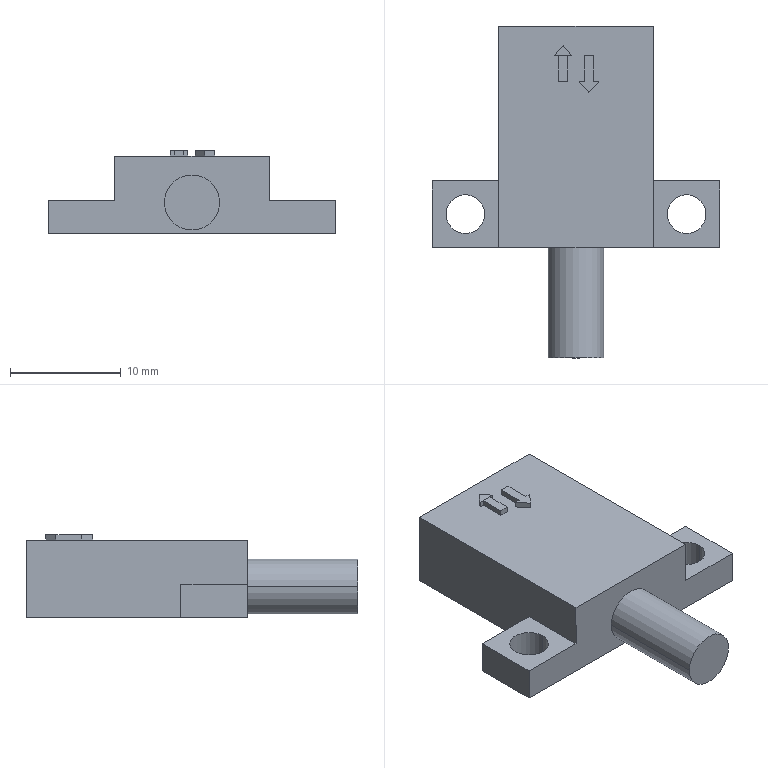Part | NX | features BREP 1 | 1 solid | 41 faces | box 26 x 30 x 7.5 mm | volume 2301 mm3 | plane 35 | cylinder 6 | commonest cylinder face diameters 3.5 x4 5 x2
STEP:
#1=CARTESIAN_POINT('',(4.,19.5,5.5));
#2=VERTEX_POINT('',#1);
#3=CARTESIAN_POINT('',(4.,19.5,1.5));
#4=VERTEX_POINT('',#3);
#5=CARTESIAN_POINT('',(4.,19.5,5.5));
#6=DIRECTION('',(0.,0.,-1.));
#7=VECTOR('',#6,1000.);
#8=LINE('',#5,#7);
#9=EDGE_CURVE('',#2,#4,#8,.T.);
#10=ORIENTED_EDGE('',*,*,#9,.T.);
#11=CARTESIAN_POINT('',(-4.,19.5,1.5));
#12=VERTEX_POINT('',#11);
#13=CARTESIAN_POINT('',(-4.,19.5,1.5));
#14=DIRECTION('',(-1.,0.,0.));
#15=VECTOR('',#14,1000.);
#16=LINE('',#13,#15);
#17=EDGE_CURVE('',#4,#12,#16,.T.);
#18=ORIENTED_EDGE('',*,*,#17,.T.);
#19=CARTESIAN_POINT('',(-4.,19.5,5.5));
#20=VERTEX_POINT('',#19);
#21=CARTESIAN_POINT('',(-4.,19.5,5.5));
#22=DIRECTION('',(0.,0.,1.));
#23=VECTOR('',#22,1000.);
#24=LINE('',#21,#23);
#25=EDGE_CURVE('',#12,#20,#24,.T.);
#26=ORIENTED_EDGE('',*,*,#25,.T.);
#27=CARTESIAN_POINT('',(-4.,19.5,5.5));
#28=DIRECTION('',(1.,0.,0.));
#29=VECTOR('',#28,1000.);
#30=LINE('',#27,#29);
#31=EDGE_CURVE('',#20,#2,#30,.T.);
#32=ORIENTED_EDGE('',*,*,#31,.T.);
#33=EDGE_LOOP('',(#10,#18,#26,#32));
#34=FACE_BOUND('',#33,.T.);
#35=CARTESIAN_POINT('',(0.,19.5,0.));
#36=DIRECTION('',(0.,-1.,0.));
#37=DIRECTION('',(0.,0.,-1.));
#38=AXIS2_PLACEMENT_3D('',#35,#36,#37);
#39=PLANE('',#38);
#40=ADVANCED_FACE('',(#34),#39,.F.);
#41=CARTESIAN_POINT('',(4.,20.,1.5));
#42=VERTEX_POINT('',#41);
#43=CARTESIAN_POINT('',(-4.,20.,1.5));
#44=VERTEX_POINT('',#43);
#45=CARTESIAN_POINT('',(-4.,20.,1.5));
#46=DIRECTION('',(-1.,0.,0.));
#47=VECTOR('',#46,1000.);
#48=LINE('',#45,#47);
#49=EDGE_CURVE('',#42,#44,#48,.T.);
#50=ORIENTED_EDGE('',*,*,#49,.T.);
#51=CARTESIAN_POINT('',(-4.,19.5,1.5));
#52=DIRECTION('',(0.,1.,0.));
#53=VECTOR('',#52,1000.);
#54=LINE('',#51,#53);
#55=EDGE_CURVE('',#12,#44,#54,.T.);
#56=ORIENTED_EDGE('',*,*,#55,.F.);
#57=ORIENTED_EDGE('',*,*,#17,.F.);
#58=CARTESIAN_POINT('',(4.,19.5,1.5));
#59=DIRECTION('',(0.,1.,0.));
#60=VECTOR('',#59,1000.);
#61=LINE('',#58,#60);
#62=EDGE_CURVE('',#4,#42,#61,.T.);
#63=ORIENTED_EDGE('',*,*,#62,.T.);
#64=EDGE_LOOP('',(#50,#56,#57,#63));
#65=FACE_BOUND('',#64,.T.);
#66=CARTESIAN_POINT('',(-4.,19.5,1.5));
#67=DIRECTION('',(0.,0.,-1.));
#68=DIRECTION('',(-1.,0.,0.));
#69=AXIS2_PLACEMENT_3D('',#66,#67,#68);
#70=PLANE('',#69);
#71=ADVANCED_FACE('',(#65),#70,.F.);
#72=CARTESIAN_POINT('',(-4.,20.,5.5));
#73=VERTEX_POINT('',#72);
#74=CARTESIAN_POINT('',(-4.,20.,5.5));
#75=DIRECTION('',(0.,0.,1.));
#76=VECTOR('',#75,1000.);
#77=LINE('',#74,#76);
#78=EDGE_CURVE('',#44,#73,#77,.T.);
#79=ORIENTED_EDGE('',*,*,#78,.T.);
#80=CARTESIAN_POINT('',(-4.,19.5,5.5));
#81=DIRECTION('',(0.,1.,0.));
#82=VECTOR('',#81,1000.);
#83=LINE('',#80,#82);
#84=EDGE_CURVE('',#20,#73,#83,.T.);
#85=ORIENTED_EDGE('',*,*,#84,.F.);
#86=ORIENTED_EDGE('',*,*,#25,.F.);
#87=ORIENTED_EDGE('',*,*,#55,.T.);
#88=EDGE_LOOP('',(#79,#85,#86,#87));
#89=FACE_BOUND('',#88,.T.);
#90=CARTESIAN_POINT('',(-4.,19.5,5.5));
#91=DIRECTION('',(-1.,0.,0.));
#92=DIRECTION('',(0.,0.,1.));
#93=AXIS2_PLACEMENT_3D('',#90,#91,#92);
#94=PLANE('',#93);
#95=ADVANCED_FACE('',(#89),#94,.F.);
#96=CARTESIAN_POINT('',(4.,20.,5.5));
#97=VERTEX_POINT('',#96);
#98=CARTESIAN_POINT('',(-4.,20.,5.5));
#99=DIRECTION('',(1.,0.,0.));
#100=VECTOR('',#99,1000.);
#101=LINE('',#98,#100);
#102=EDGE_CURVE('',#73,#97,#101,.T.);
#103=ORIENTED_EDGE('',*,*,#102,.T.);
#104=CARTESIAN_POINT('',(4.,19.5,5.5));
#105=DIRECTION('',(0.,1.,0.));
#106=VECTOR('',#105,1000.);
#107=LINE('',#104,#106);
#108=EDGE_CURVE('',#2,#97,#107,.T.);
#109=ORIENTED_EDGE('',*,*,#108,.F.);
#110=ORIENTED_EDGE('',*,*,#31,.F.);
#111=ORIENTED_EDGE('',*,*,#84,.T.);
#112=EDGE_LOOP('',(#103,#109,#110,#111));
#113=FACE_BOUND('',#112,.T.);
#114=CARTESIAN_POINT('',(-4.,19.5,5.5));
#115=DIRECTION('',(0.,0.,1.));
#116=DIRECTION('',(1.,0.,0.));
#117=AXIS2_PLACEMENT_3D('',#114,#115,#116);
#118=PLANE('',#117);
#119=ADVANCED_FACE('',(#113),#118,.F.);
#120=CARTESIAN_POINT('',(4.,20.,5.5));
#121=DIRECTION('',(0.,0.,-1.));
#122=VECTOR('',#121,1000.);
#123=LINE('',#120,#122);
#124=EDGE_CURVE('',#97,#42,#123,.T.);
#125=ORIENTED_EDGE('',*,*,#124,.T.);
#126=ORIENTED_EDGE('',*,*,#62,.F.);
#127=ORIENTED_EDGE('',*,*,#9,.F.);
#128=ORIENTED_EDGE('',*,*,#108,.T.);
#129=EDGE_LOOP('',(#125,#126,#127,#128));
#130=FACE_BOUND('',#129,.T.);
#131=CARTESIAN_POINT('',(4.,19.5,5.5));
#132=DIRECTION('',(1.,0.,0.));
#133=DIRECTION('',(0.,0.,-1.));
#134=AXIS2_PLACEMENT_3D('',#131,#132,#133);
#135=PLANE('',#134);
#136=ADVANCED_FACE('',(#130),#135,.F.);
#137=CARTESIAN_POINT('',(-2.5,-10.,2.8));
#138=VERTEX_POINT('',#137);
#139=CARTESIAN_POINT('',(2.5,-10.,2.8));
#140=VERTEX_POINT('',#139);
#141=CARTESIAN_POINT('',(0.,-10.,2.8));
#142=DIRECTION('',(0.,-1.,0.));
#143=DIRECTION('',(1.,0.,0.));
#144=AXIS2_PLACEMENT_3D('',#141,#142,#143);
#145=CIRCLE('',#144,2.5);
#146=EDGE_CURVE('',#138,#140,#145,.T.);
#147=ORIENTED_EDGE('',*,*,#146,.T.);
#148=CARTESIAN_POINT('',(0.,-10.,2.8));
#149=DIRECTION('',(0.,-1.,0.));
#150=DIRECTION('',(1.,0.,0.));
#151=AXIS2_PLACEMENT_3D('',#148,#149,#150);
#152=CIRCLE('',#151,2.5);
#153=EDGE_CURVE('',#140,#138,#152,.T.);
#154=ORIENTED_EDGE('',*,*,#153,.T.);
#155=EDGE_LOOP('',(#147,#154));
#156=FACE_BOUND('',#155,.T.);
#157=CARTESIAN_POINT('',(0.,-10.,2.8));
#158=DIRECTION('',(0.,-1.,0.));
#159=DIRECTION('',(1.,0.,0.));
#160=AXIS2_PLACEMENT_3D('',#157,#158,#159);
#161=PLANE('',#160);
#162=ADVANCED_FACE('',(#156),#161,.T.);
#163=CARTESIAN_POINT('',(2.5,0.,2.8));
#164=VERTEX_POINT('',#163);
#165=CARTESIAN_POINT('',(2.5,-10.,2.8));
#166=DIRECTION('',(0.,1.,0.));
#167=VECTOR('',#166,1000.);
#168=LINE('',#165,#167);
#169=EDGE_CURVE('',#140,#164,#168,.T.);
#170=ORIENTED_EDGE('',*,*,#169,.F.);
#171=ORIENTED_EDGE('',*,*,#146,.F.);
#172=CARTESIAN_POINT('',(-2.5,0.,2.8));
#173=VERTEX_POINT('',#172);
#174=CARTESIAN_POINT('',(-2.5,-10.,2.8));
#175=DIRECTION('',(0.,1.,0.));
#176=VECTOR('',#175,1000.);
#177=LINE('',#174,#176);
#178=EDGE_CURVE('',#138,#173,#177,.T.);
#179=ORIENTED_EDGE('',*,*,#178,.T.);
#180=CARTESIAN_POINT('',(0.,0.,2.8));
#181=DIRECTION('',(0.,-1.,0.));
#182=DIRECTION('',(-1.,0.,0.));
#183=AXIS2_PLACEMENT_3D('',#180,#181,#182);
#184=CIRCLE('',#183,2.5);
#185=EDGE_CURVE('',#173,#164,#184,.T.);
#186=ORIENTED_EDGE('',*,*,#185,.T.);
#187=EDGE_LOOP('',(#170,#171,#179,#186));
#188=FACE_BOUND('',#187,.T.);
#189=CARTESIAN_POINT('',(0.,-10.,2.8));
#190=DIRECTION('',(0.,1.,0.));
#191=DIRECTION('',(-1.,0.,0.));
#192=AXIS2_PLACEMENT_3D('',#189,#190,#191);
#193=CYLINDRICAL_SURFACE('',#192,2.5);
#194=ADVANCED_FACE('',(#188),#193,.T.);
#195=CARTESIAN_POINT('',(-11.75,3.,3.));
#196=VERTEX_POINT('',#195);
#197=CARTESIAN_POINT('',(-11.75,3.,0.));
#198=VERTEX_POINT('',#197);
#199=CARTESIAN_POINT('',(-11.75,3.,3.));
#200=DIRECTION('',(0.,0.,1.));
#201=VECTOR('',#200,1000.);
#202=LINE('',#199,#201);
#203=EDGE_CURVE('',#196,#198,#202,.F.);
#204=ORIENTED_EDGE('',*,*,#203,.T.);
#205=CARTESIAN_POINT('',(-8.25,3.,0.));
#206=VERTEX_POINT('',#205);
#207=CARTESIAN_POINT('',(-10.,3.,0.));
#208=DIRECTION('',(0.,0.,1.));
#209=DIRECTION('',(1.,0.,0.));
#210=AXIS2_PLACEMENT_3D('',#207,#208,#209);
#211=CIRCLE('',#210,1.75);
#212=EDGE_CURVE('',#206,#198,#211,.T.);
#213=ORIENTED_EDGE('',*,*,#212,.F.);
#214=CARTESIAN_POINT('',(-8.25,3.,3.));
#215=VERTEX_POINT('',#214);
#216=CARTESIAN_POINT('',(-8.25,3.,3.));
#217=DIRECTION('',(0.,0.,1.));
#218=VECTOR('',#217,1000.);
#219=LINE('',#216,#218);
#220=EDGE_CURVE('',#215,#206,#219,.F.);
#221=ORIENTED_EDGE('',*,*,#220,.F.);
#222=CARTESIAN_POINT('',(-10.,3.,3.));
#223=DIRECTION('',(0.,0.,1.));
#224=DIRECTION('',(1.,0.,0.));
#225=AXIS2_PLACEMENT_3D('',#222,#223,#224);
#226=CIRCLE('',#225,1.75);
#227=EDGE_CURVE('',#215,#196,#226,.T.);
#228=ORIENTED_EDGE('',*,*,#227,.T.);
#229=EDGE_LOOP('',(#204,#213,#221,#228));
#230=FACE_BOUND('',#229,.T.);
#231=CARTESIAN_POINT('',(-10.,3.,3.));
#232=DIRECTION('',(0.,0.,1.));
#233=DIRECTION('',(1.,0.,0.));
#234=AXIS2_PLACEMENT_3D('',#231,#232,#233);
#235=CYLINDRICAL_SURFACE('',#234,1.75);
#236=ADVANCED_FACE('',(#230),#235,.F.);
#237=CARTESIAN_POINT('',(8.25,3.,3.));
#238=VERTEX_POINT('',#237);
#239=CARTESIAN_POINT('',(8.25,3.,0.));
#240=VERTEX_POINT('',#239);
#241=CARTESIAN_POINT('',(8.25,3.,3.));
#242=DIRECTION('',(0.,0.,1.));
#243=VECTOR('',#242,1000.);
#244=LINE('',#241,#243);
#245=EDGE_CURVE('',#238,#240,#244,.F.);
#246=ORIENTED_EDGE('',*,*,#245,.T.);
#247=CARTESIAN_POINT('',(11.75,3.,0.));
#248=VERTEX_POINT('',#247);
#249=CARTESIAN_POINT('',(10.,3.,0.));
#250=DIRECTION('',(0.,0.,1.));
#251=DIRECTION('',(1.,0.,0.));
#252=AXIS2_PLACEMENT_3D('',#249,#250,#251);
#253=CIRCLE('',#252,1.75);
#254=EDGE_CURVE('',#248,#240,#253,.T.);
#255=ORIENTED_EDGE('',*,*,#254,.F.);
#256=CARTESIAN_POINT('',(11.75,3.,3.));
#257=VERTEX_POINT('',#256);
#258=CARTESIAN_POINT('',(11.75,3.,3.));
#259=DIRECTION('',(0.,0.,1.));
#260=VECTOR('',#259,1000.);
#261=LINE('',#258,#260);
#262=EDGE_CURVE('',#257,#248,#261,.F.);
#263=ORIENTED_EDGE('',*,*,#262,.F.);
#264=CARTESIAN_POINT('',(10.,3.,3.));
#265=DIRECTION('',(0.,0.,1.));
#266=DIRECTION('',(1.,0.,0.));
#267=AXIS2_PLACEMENT_3D('',#264,#265,#266);
#268=CIRCLE('',#267,1.75);
#269=EDGE_CURVE('',#257,#238,#268,.T.);
#270=ORIENTED_EDGE('',*,*,#269,.T.);
#271=EDGE_LOOP('',(#246,#255,#263,#270));
#272=FACE_BOUND('',#271,.T.);
#273=CARTESIAN_POINT('',(10.,3.,3.));
#274=DIRECTION('',(0.,0.,1.));
#275=DIRECTION('',(1.,0.,0.));
#276=AXIS2_PLACEMENT_3D('',#273,#274,#275);
#277=CYLINDRICAL_SURFACE('',#276,1.75);
#278=ADVANCED_FACE('',(#272),#277,.F.);
#279=CARTESIAN_POINT('',(1.592,17.295,7.5));
#280=VERTEX_POINT('',#279);
#281=CARTESIAN_POINT('',(1.592,15.02,7.5));
#282=VERTEX_POINT('',#281);
#283=CARTESIAN_POINT('',(1.592,0.,7.5));
#284=DIRECTION('',(0.,-1.,0.));
#285=VECTOR('',#284,1000.);
#286=LINE('',#283,#285);
#287=EDGE_CURVE('',#280,#282,#286,.T.);
#288=ORIENTED_EDGE('',*,*,#287,.F.);
#289=CARTESIAN_POINT('',(0.7557,17.295,7.5));
#290=VERTEX_POINT('',#289);
#291=CARTESIAN_POINT('',(0.,17.295,7.5));
#292=DIRECTION('',(1.,0.,0.));
#293=VECTOR('',#292,1000.);
#294=LINE('',#291,#293);
#295=EDGE_CURVE('',#290,#280,#294,.T.);
#296=ORIENTED_EDGE('',*,*,#295,.F.);
#297=CARTESIAN_POINT('',(0.7557,15.02,7.5));
#298=VERTEX_POINT('',#297);
#299=CARTESIAN_POINT('',(0.7557,0.,7.5));
#300=DIRECTION('',(0.,-1.,0.));
#301=VECTOR('',#300,1000.);
#302=LINE('',#299,#301);
#303=EDGE_CURVE('',#290,#298,#302,.T.);
#304=ORIENTED_EDGE('',*,*,#303,.T.);
#305=CARTESIAN_POINT('',(0.2749,15.02,7.5));
#306=VERTEX_POINT('',#305);
#307=CARTESIAN_POINT('',(0.,15.02,7.5));
#308=DIRECTION('',(1.,0.,0.));
#309=VECTOR('',#308,1000.);
#310=LINE('',#307,#309);
#311=EDGE_CURVE('',#306,#298,#310,.T.);
#312=ORIENTED_EDGE('',*,*,#311,.F.);
#313=CARTESIAN_POINT('',(1.174,13.95,7.5));
#314=VERTEX_POINT('',#313);
#315=CARTESIAN_POINT('',(7.559,6.351,7.5));
#316=DIRECTION('',(-0.6433,0.7656,0.));
#317=VECTOR('',#316,1000.);
#318=LINE('',#315,#317);
#319=EDGE_CURVE('',#314,#306,#318,.T.);
#320=ORIENTED_EDGE('',*,*,#319,.F.);
#321=CARTESIAN_POINT('',(2.073,15.02,7.5));
#322=VERTEX_POINT('',#321);
#323=CARTESIAN_POINT('',(-6.183,5.195,7.5));
#324=DIRECTION('',(-0.6433,-0.7656,0.));
#325=VECTOR('',#324,1000.);
#326=LINE('',#323,#325);
#327=EDGE_CURVE('',#322,#314,#326,.T.);
#328=ORIENTED_EDGE('',*,*,#327,.F.);
#329=CARTESIAN_POINT('',(0.,15.02,7.5));
#330=DIRECTION('',(1.,0.,0.));
#331=VECTOR('',#330,1000.);
#332=LINE('',#329,#331);
#333=EDGE_CURVE('',#282,#322,#332,.T.);
#334=ORIENTED_EDGE('',*,*,#333,.F.);
#335=EDGE_LOOP('',(#288,#296,#304,#312,#320,#328,#334));
#336=FACE_BOUND('',#335,.T.);
#337=CARTESIAN_POINT('',(0.,0.,7.5));
#338=DIRECTION('',(0.,0.,1.));
#339=DIRECTION('',(1.,0.,0.));
#340=AXIS2_PLACEMENT_3D('',#337,#338,#339);
#341=PLANE('',#340);
#342=ADVANCED_FACE('',(#336),#341,.T.);
#343=CARTESIAN_POINT('',(1.592,15.02,7.));
#344=VERTEX_POINT('',#343);
#345=CARTESIAN_POINT('',(2.073,15.02,7.));
#346=VERTEX_POINT('',#345);
#347=CARTESIAN_POINT('',(0.,15.02,7.));
#348=DIRECTION('',(1.,0.,0.));
#349=VECTOR('',#348,1000.);
#350=LINE('',#347,#349);
#351=EDGE_CURVE('',#344,#346,#350,.T.);
#352=ORIENTED_EDGE('',*,*,#351,.F.);
#353=CARTESIAN_POINT('',(1.592,15.02,7.5));
#354=DIRECTION('',(0.,0.,-1.));
#355=VECTOR('',#354,1000.);
#356=LINE('',#353,#355);
#357=EDGE_CURVE('',#282,#344,#356,.T.);
#358=ORIENTED_EDGE('',*,*,#357,.F.);
#359=ORIENTED_EDGE('',*,*,#333,.T.);
#360=CARTESIAN_POINT('',(2.073,15.02,7.5));
#361=DIRECTION('',(0.,0.,-1.));
#362=VECTOR('',#361,1000.);
#363=LINE('',#360,#362);
#364=EDGE_CURVE('',#322,#346,#363,.T.);
#365=ORIENTED_EDGE('',*,*,#364,.T.);
#366=EDGE_LOOP('',(#352,#358,#359,#365));
#367=FACE_BOUND('',#366,.T.);
#368=CARTESIAN_POINT('',(0.,15.02,7.5));
#369=DIRECTION('',(0.,1.,0.));
#370=DIRECTION('',(0.,0.,1.));
#371=AXIS2_PLACEMENT_3D('',#368,#369,#370);
#372=PLANE('',#371);
#373=ADVANCED_FACE('',(#367),#372,.T.);
#374=CARTESIAN_POINT('',(1.174,13.95,7.));
#375=VERTEX_POINT('',#374);
#376=CARTESIAN_POINT('',(-6.183,5.195,7.));
#377=DIRECTION('',(-0.6433,-0.7656,0.));
#378=VECTOR('',#377,1000.);
#379=LINE('',#376,#378);
#380=EDGE_CURVE('',#346,#375,#379,.T.);
#381=ORIENTED_EDGE('',*,*,#380,.F.);
#382=ORIENTED_EDGE('',*,*,#364,.F.);
#383=ORIENTED_EDGE('',*,*,#327,.T.);
#384=CARTESIAN_POINT('',(1.174,13.95,7.5));
#385=DIRECTION('',(0.,0.,-1.));
#386=VECTOR('',#385,1000.);
#387=LINE('',#384,#386);
#388=EDGE_CURVE('',#314,#375,#387,.T.);
#389=ORIENTED_EDGE('',*,*,#388,.T.);
#390=EDGE_LOOP('',(#381,#382,#383,#389));
#391=FACE_BOUND('',#390,.T.);
#392=CARTESIAN_POINT('',(-6.183,5.195,7.5));
#393=DIRECTION('',(0.7656,-0.6433,0.));
#394=DIRECTION('',(0.6433,0.7656,0.));
#395=AXIS2_PLACEMENT_3D('',#392,#393,#394);
#396=PLANE('',#395);
#397=ADVANCED_FACE('',(#391),#396,.T.);
#398=CARTESIAN_POINT('',(0.2749,15.02,7.));
#399=VERTEX_POINT('',#398);
#400=CARTESIAN_POINT('',(7.559,6.351,7.));
#401=DIRECTION('',(-0.6433,0.7656,0.));
#402=VECTOR('',#401,1000.);
#403=LINE('',#400,#402);
#404=EDGE_CURVE('',#375,#399,#403,.T.);
#405=ORIENTED_EDGE('',*,*,#404,.F.);
#406=ORIENTED_EDGE('',*,*,#388,.F.);
#407=ORIENTED_EDGE('',*,*,#319,.T.);
#408=CARTESIAN_POINT('',(0.2749,15.02,7.5));
#409=DIRECTION('',(0.,0.,-1.));
#410=VECTOR('',#409,1000.);
#411=LINE('',#408,#410);
#412=EDGE_CURVE('',#306,#399,#411,.T.);
#413=ORIENTED_EDGE('',*,*,#412,.T.);
#414=EDGE_LOOP('',(#405,#406,#407,#413));
#415=FACE_BOUND('',#414,.T.);
#416=CARTESIAN_POINT('',(7.559,6.351,7.5));
#417=DIRECTION('',(-0.7656,-0.6433,0.));
#418=DIRECTION('',(0.6433,-0.7656,0.));
#419=AXIS2_PLACEMENT_3D('',#416,#417,#418);
#420=PLANE('',#419);
#421=ADVANCED_FACE('',(#415),#420,.T.);
#422=CARTESIAN_POINT('',(0.7557,15.02,7.));
#423=VERTEX_POINT('',#422);
#424=CARTESIAN_POINT('',(0.,15.02,7.));
#425=DIRECTION('',(1.,0.,0.));
#426=VECTOR('',#425,1000.);
#427=LINE('',#424,#426);
#428=EDGE_CURVE('',#399,#423,#427,.T.);
#429=ORIENTED_EDGE('',*,*,#428,.F.);
#430=ORIENTED_EDGE('',*,*,#412,.F.);
#431=ORIENTED_EDGE('',*,*,#311,.T.);
#432=CARTESIAN_POINT('',(0.7557,15.02,7.5));
#433=DIRECTION('',(0.,0.,-1.));
#434=VECTOR('',#433,1000.);
#435=LINE('',#432,#434);
#436=EDGE_CURVE('',#298,#423,#435,.T.);
#437=ORIENTED_EDGE('',*,*,#436,.T.);
#438=EDGE_LOOP('',(#429,#430,#431,#437));
#439=FACE_BOUND('',#438,.T.);
#440=CARTESIAN_POINT('',(0.,15.02,7.5));
#441=DIRECTION('',(0.,1.,0.));
#442=DIRECTION('',(0.,0.,1.));
#443=AXIS2_PLACEMENT_3D('',#440,#441,#442);
#444=PLANE('',#443);
#445=ADVANCED_FACE('',(#439),#444,.T.);
#446=CARTESIAN_POINT('',(0.7557,17.295,7.));
#447=VERTEX_POINT('',#446);
#448=CARTESIAN_POINT('',(0.7557,0.,7.));
#449=DIRECTION('',(0.,-1.,0.));
#450=VECTOR('',#449,1000.);
#451=LINE('',#448,#450);
#452=EDGE_CURVE('',#447,#423,#451,.T.);
#453=ORIENTED_EDGE('',*,*,#452,.T.);
#454=ORIENTED_EDGE('',*,*,#436,.F.);
#455=ORIENTED_EDGE('',*,*,#303,.F.);
#456=CARTESIAN_POINT('',(0.7557,17.295,7.5));
#457=DIRECTION('',(0.,0.,-1.));
#458=VECTOR('',#457,1000.);
#459=LINE('',#456,#458);
#460=EDGE_CURVE('',#290,#447,#459,.T.);
#461=ORIENTED_EDGE('',*,*,#460,.T.);
#462=EDGE_LOOP('',(#453,#454,#455,#461));
#463=FACE_BOUND('',#462,.T.);
#464=CARTESIAN_POINT('',(0.7557,0.,7.5));
#465=DIRECTION('',(1.,0.,0.));
#466=DIRECTION('',(0.,1.,0.));
#467=AXIS2_PLACEMENT_3D('',#464,#465,#466);
#468=PLANE('',#467);
#469=ADVANCED_FACE('',(#463),#468,.F.);
#470=CARTESIAN_POINT('',(1.592,17.295,7.));
#471=VERTEX_POINT('',#470);
#472=CARTESIAN_POINT('',(0.,17.295,7.));
#473=DIRECTION('',(1.,0.,0.));
#474=VECTOR('',#473,1000.);
#475=LINE('',#472,#474);
#476=EDGE_CURVE('',#447,#471,#475,.T.);
#477=ORIENTED_EDGE('',*,*,#476,.F.);
#478=ORIENTED_EDGE('',*,*,#460,.F.);
#479=ORIENTED_EDGE('',*,*,#295,.T.);
#480=CARTESIAN_POINT('',(1.592,17.295,7.5));
#481=DIRECTION('',(0.,0.,-1.));
#482=VECTOR('',#481,1000.);
#483=LINE('',#480,#482);
#484=EDGE_CURVE('',#280,#471,#483,.T.);
#485=ORIENTED_EDGE('',*,*,#484,.T.);
#486=EDGE_LOOP('',(#477,#478,#479,#485));
#487=FACE_BOUND('',#486,.T.);
#488=CARTESIAN_POINT('',(0.,17.295,7.5));
#489=DIRECTION('',(0.,1.,0.));
#490=DIRECTION('',(-1.,0.,0.));
#491=AXIS2_PLACEMENT_3D('',#488,#489,#490);
#492=PLANE('',#491);
#493=ADVANCED_FACE('',(#487),#492,.T.);
#494=CARTESIAN_POINT('',(1.592,0.,7.));
#495=DIRECTION('',(0.,-1.,0.));
#496=VECTOR('',#495,1000.);
#497=LINE('',#494,#496);
#498=EDGE_CURVE('',#471,#344,#497,.T.);
#499=ORIENTED_EDGE('',*,*,#498,.F.);
#500=ORIENTED_EDGE('',*,*,#484,.F.);
#501=ORIENTED_EDGE('',*,*,#287,.T.);
#502=ORIENTED_EDGE('',*,*,#357,.T.);
#503=EDGE_LOOP('',(#499,#500,#501,#502));
#504=FACE_BOUND('',#503,.T.);
#505=CARTESIAN_POINT('',(1.592,0.,7.5));
#506=DIRECTION('',(1.,0.,0.));
#507=DIRECTION('',(0.,0.,-1.));
#508=AXIS2_PLACEMENT_3D('',#505,#506,#507);
#509=PLANE('',#508);
#510=ADVANCED_FACE('',(#504),#509,.T.);
#511=CARTESIAN_POINT('',(-1.592,15.02,7.5));
#512=VERTEX_POINT('',#511);
#513=CARTESIAN_POINT('',(-0.7557,15.02,7.5));
#514=VERTEX_POINT('',#513);
#515=CARTESIAN_POINT('',(0.,15.02,7.5));
#516=DIRECTION('',(1.,0.,0.));
#517=VECTOR('',#516,1000.);
#518=LINE('',#515,#517);
#519=EDGE_CURVE('',#512,#514,#518,.T.);
#520=ORIENTED_EDGE('',*,*,#519,.T.);
#521=CARTESIAN_POINT('',(-0.7557,17.295,7.5));
#522=VERTEX_POINT('',#521);
#523=CARTESIAN_POINT('',(-0.7557,0.,7.5));
#524=DIRECTION('',(0.,1.,0.));
#525=VECTOR('',#524,1000.);
#526=LINE('',#523,#525);
#527=EDGE_CURVE('',#514,#522,#526,.T.);
#528=ORIENTED_EDGE('',*,*,#527,.T.);
#529=CARTESIAN_POINT('',(-1.592,17.295,7.5));
#530=VERTEX_POINT('',#529);
#531=CARTESIAN_POINT('',(0.,17.295,7.5));
#532=DIRECTION('',(1.,0.,0.));
#533=VECTOR('',#532,1000.);
#534=LINE('',#531,#533);
#535=EDGE_CURVE('',#530,#522,#534,.T.);
#536=ORIENTED_EDGE('',*,*,#535,.F.);
#537=CARTESIAN_POINT('',(-1.592,0.,7.5));
#538=DIRECTION('',(0.,1.,0.));
#539=VECTOR('',#538,1000.);
#540=LINE('',#537,#539);
#541=EDGE_CURVE('',#512,#530,#540,.T.);
#542=ORIENTED_EDGE('',*,*,#541,.F.);
#543=EDGE_LOOP('',(#520,#528,#536,#542));
#544=FACE_BOUND('',#543,.T.);
#545=CARTESIAN_POINT('',(0.,0.,7.5));
#546=DIRECTION('',(0.,0.,1.));
#547=DIRECTION('',(1.,0.,0.));
#548=AXIS2_PLACEMENT_3D('',#545,#546,#547);
#549=PLANE('',#548);
#550=ADVANCED_FACE('',(#544),#549,.T.);
#551=CARTESIAN_POINT('',(-1.592,15.02,7.));
#552=VERTEX_POINT('',#551);
#553=CARTESIAN_POINT('',(-1.592,17.295,7.));
#554=VERTEX_POINT('',#553);
#555=CARTESIAN_POINT('',(-1.592,0.,7.));
#556=DIRECTION('',(0.,1.,0.));
#557=VECTOR('',#556,1000.);
#558=LINE('',#555,#557);
#559=EDGE_CURVE('',#552,#554,#558,.T.);
#560=ORIENTED_EDGE('',*,*,#559,.F.);
#561=CARTESIAN_POINT('',(-1.592,15.02,7.5));
#562=DIRECTION('',(0.,0.,-1.));
#563=VECTOR('',#562,1000.);
#564=LINE('',#561,#563);
#565=EDGE_CURVE('',#512,#552,#564,.T.);
#566=ORIENTED_EDGE('',*,*,#565,.F.);
#567=ORIENTED_EDGE('',*,*,#541,.T.);
#568=CARTESIAN_POINT('',(-1.592,17.295,7.5));
#569=DIRECTION('',(0.,0.,-1.));
#570=VECTOR('',#569,1000.);
#571=LINE('',#568,#570);
#572=EDGE_CURVE('',#530,#554,#571,.T.);
#573=ORIENTED_EDGE('',*,*,#572,.T.);
#574=EDGE_LOOP('',(#560,#566,#567,#573));
#575=FACE_BOUND('',#574,.T.);
#576=CARTESIAN_POINT('',(-1.592,0.,7.5));
#577=DIRECTION('',(-1.,0.,0.));
#578=DIRECTION('',(0.,0.,1.));
#579=AXIS2_PLACEMENT_3D('',#576,#577,#578);
#580=PLANE('',#579);
#581=ADVANCED_FACE('',(#575),#580,.T.);
#582=CARTESIAN_POINT('',(-0.7557,17.295,7.));
#583=VERTEX_POINT('',#582);
#584=CARTESIAN_POINT('',(0.,17.295,7.));
#585=DIRECTION('',(1.,0.,0.));
#586=VECTOR('',#585,1000.);
#587=LINE('',#584,#586);
#588=EDGE_CURVE('',#554,#583,#587,.T.);
#589=ORIENTED_EDGE('',*,*,#588,.F.);
#590=ORIENTED_EDGE('',*,*,#572,.F.);
#591=ORIENTED_EDGE('',*,*,#535,.T.);
#592=CARTESIAN_POINT('',(-0.7557,17.295,7.5));
#593=DIRECTION('',(0.,0.,-1.));
#594=VECTOR('',#593,1000.);
#595=LINE('',#592,#594);
#596=EDGE_CURVE('',#522,#583,#595,.T.);
#597=ORIENTED_EDGE('',*,*,#596,.T.);
#598=EDGE_LOOP('',(#589,#590,#591,#597));
#599=FACE_BOUND('',#598,.T.);
#600=CARTESIAN_POINT('',(0.,17.295,7.5));
#601=DIRECTION('',(0.,1.,0.));
#602=DIRECTION('',(0.,0.,1.));
#603=AXIS2_PLACEMENT_3D('',#600,#601,#602);
#604=PLANE('',#603);
#605=ADVANCED_FACE('',(#599),#604,.T.);
#606=CARTESIAN_POINT('',(-0.7557,15.02,7.));
#607=VERTEX_POINT('',#606);
#608=CARTESIAN_POINT('',(-0.7557,0.,7.));
#609=DIRECTION('',(0.,1.,0.));
#610=VECTOR('',#609,1000.);
#611=LINE('',#608,#610);
#612=EDGE_CURVE('',#607,#583,#611,.T.);
#613=ORIENTED_EDGE('',*,*,#612,.T.);
#614=ORIENTED_EDGE('',*,*,#596,.F.);
#615=ORIENTED_EDGE('',*,*,#527,.F.);
#616=CARTESIAN_POINT('',(-0.7557,15.02,7.5));
#617=DIRECTION('',(0.,0.,-1.));
#618=VECTOR('',#617,1000.);
#619=LINE('',#616,#618);
#620=EDGE_CURVE('',#514,#607,#619,.T.);
#621=ORIENTED_EDGE('',*,*,#620,.T.);
#622=EDGE_LOOP('',(#613,#614,#615,#621));
#623=FACE_BOUND('',#622,.T.);
#624=CARTESIAN_POINT('',(-0.7557,0.,7.5));
#625=DIRECTION('',(-1.,0.,0.));
#626=DIRECTION('',(0.,-1.,0.));
#627=AXIS2_PLACEMENT_3D('',#624,#625,#626);
#628=PLANE('',#627);
#629=ADVANCED_FACE('',(#623),#628,.F.);
#630=CARTESIAN_POINT('',(0.,15.02,7.));
#631=DIRECTION('',(1.,0.,0.));
#632=VECTOR('',#631,1000.);
#633=LINE('',#630,#632);
#634=EDGE_CURVE('',#552,#607,#633,.T.);
#635=ORIENTED_EDGE('',*,*,#634,.T.);
#636=ORIENTED_EDGE('',*,*,#620,.F.);
#637=ORIENTED_EDGE('',*,*,#519,.F.);
#638=ORIENTED_EDGE('',*,*,#565,.T.);
#639=EDGE_LOOP('',(#635,#636,#637,#638));
#640=FACE_BOUND('',#639,.T.);
#641=CARTESIAN_POINT('',(0.,15.02,7.5));
#642=DIRECTION('',(0.,1.,0.));
#643=DIRECTION('',(0.,0.,1.));
#644=AXIS2_PLACEMENT_3D('',#641,#642,#643);
#645=PLANE('',#644);
#646=ADVANCED_FACE('',(#640),#645,.F.);
#647=CARTESIAN_POINT('',(-0.3905,17.301,7.5));
#648=VERTEX_POINT('',#647);
#649=CARTESIAN_POINT('',(-1.957,17.301,7.5));
#650=VERTEX_POINT('',#649);
#651=CARTESIAN_POINT('',(0.,17.301,7.5));
#652=DIRECTION('',(-1.,0.,0.));
#653=VECTOR('',#652,1000.);
#654=LINE('',#651,#653);
#655=EDGE_CURVE('',#648,#650,#654,.T.);
#656=ORIENTED_EDGE('',*,*,#655,.F.);
#657=CARTESIAN_POINT('',(-1.174,18.21,7.5));
#658=VERTEX_POINT('',#657);
#659=CARTESIAN_POINT('',(8.333,7.186,7.5));
#660=DIRECTION('',(0.6531,-0.7573,0.));
#661=VECTOR('',#660,1000.);
#662=LINE('',#659,#661);
#663=EDGE_CURVE('',#658,#648,#662,.T.);
#664=ORIENTED_EDGE('',*,*,#663,.F.);
#665=CARTESIAN_POINT('',(-9.679,8.347,7.5));
#666=DIRECTION('',(0.6531,0.7573,0.));
#667=VECTOR('',#666,1000.);
#668=LINE('',#665,#667);
#669=EDGE_CURVE('',#650,#658,#668,.T.);
#670=ORIENTED_EDGE('',*,*,#669,.F.);
#671=EDGE_LOOP('',(#656,#664,#670));
#672=FACE_BOUND('',#671,.T.);
#673=CARTESIAN_POINT('',(0.,0.,7.5));
#674=DIRECTION('',(0.,0.,1.));
#675=DIRECTION('',(1.,0.,0.));
#676=AXIS2_PLACEMENT_3D('',#673,#674,#675);
#677=PLANE('',#676);
#678=ADVANCED_FACE('',(#672),#677,.T.);
#679=CARTESIAN_POINT('',(-1.957,17.301,7.));
#680=VERTEX_POINT('',#679);
#681=CARTESIAN_POINT('',(-1.174,18.21,7.));
#682=VERTEX_POINT('',#681);
#683=CARTESIAN_POINT('',(-9.679,8.347,7.));
#684=DIRECTION('',(0.6531,0.7573,0.));
#685=VECTOR('',#684,1000.);
#686=LINE('',#683,#685);
#687=EDGE_CURVE('',#680,#682,#686,.T.);
#688=ORIENTED_EDGE('',*,*,#687,.F.);
#689=CARTESIAN_POINT('',(-1.957,17.301,7.5));
#690=DIRECTION('',(0.,0.,-1.));
#691=VECTOR('',#690,1000.);
#692=LINE('',#689,#691);
#693=EDGE_CURVE('',#650,#680,#692,.T.);
#694=ORIENTED_EDGE('',*,*,#693,.F.);
#695=ORIENTED_EDGE('',*,*,#669,.T.);
#696=CARTESIAN_POINT('',(-1.174,18.21,7.5));
#697=DIRECTION('',(0.,0.,-1.));
#698=VECTOR('',#697,1000.);
#699=LINE('',#696,#698);
#700=EDGE_CURVE('',#658,#682,#699,.T.);
#701=ORIENTED_EDGE('',*,*,#700,.T.);
#702=EDGE_LOOP('',(#688,#694,#695,#701));
#703=FACE_BOUND('',#702,.T.);
#704=CARTESIAN_POINT('',(-9.679,8.347,7.5));
#705=DIRECTION('',(-0.7573,0.6531,0.));
#706=DIRECTION('',(-0.6531,-0.7573,0.));
#707=AXIS2_PLACEMENT_3D('',#704,#705,#706);
#708=PLANE('',#707);
#709=ADVANCED_FACE('',(#703),#708,.T.);
#710=CARTESIAN_POINT('',(-0.3905,17.301,7.));
#711=VERTEX_POINT('',#710);
#712=CARTESIAN_POINT('',(8.333,7.186,7.));
#713=DIRECTION('',(0.6531,-0.7573,0.));
#714=VECTOR('',#713,1000.);
#715=LINE('',#712,#714);
#716=EDGE_CURVE('',#682,#711,#715,.T.);
#717=ORIENTED_EDGE('',*,*,#716,.F.);
#718=ORIENTED_EDGE('',*,*,#700,.F.);
#719=ORIENTED_EDGE('',*,*,#663,.T.);
#720=CARTESIAN_POINT('',(-0.3905,17.301,7.5));
#721=DIRECTION('',(0.,0.,-1.));
#722=VECTOR('',#721,1000.);
#723=LINE('',#720,#722);
#724=EDGE_CURVE('',#648,#711,#723,.T.);
#725=ORIENTED_EDGE('',*,*,#724,.T.);
#726=EDGE_LOOP('',(#717,#718,#719,#725));
#727=FACE_BOUND('',#726,.T.);
#728=CARTESIAN_POINT('',(8.333,7.186,7.5));
#729=DIRECTION('',(0.7573,0.6531,0.));
#730=DIRECTION('',(-0.6531,0.7573,0.));
#731=AXIS2_PLACEMENT_3D('',#728,#729,#730);
#732=PLANE('',#731);
#733=ADVANCED_FACE('',(#727),#732,.T.);
#734=CARTESIAN_POINT('',(0.,17.301,7.));
#735=DIRECTION('',(-1.,0.,0.));
#736=VECTOR('',#735,1000.);
#737=LINE('',#734,#736);
#738=EDGE_CURVE('',#711,#680,#737,.T.);
#739=ORIENTED_EDGE('',*,*,#738,.F.);
#740=ORIENTED_EDGE('',*,*,#724,.F.);
#741=ORIENTED_EDGE('',*,*,#655,.T.);
#742=ORIENTED_EDGE('',*,*,#693,.T.);
#743=EDGE_LOOP('',(#739,#740,#741,#742));
#744=FACE_BOUND('',#743,.T.);
#745=CARTESIAN_POINT('',(0.,17.301,7.5));
#746=DIRECTION('',(0.,-1.,0.));
#747=DIRECTION('',(0.,0.,-1.));
#748=AXIS2_PLACEMENT_3D('',#745,#746,#747);
#749=PLANE('',#748);
#750=ADVANCED_FACE('',(#744),#749,.T.);
#751=CARTESIAN_POINT('',(13.,6.,3.));
#752=VERTEX_POINT('',#751);
#753=CARTESIAN_POINT('',(13.,0.,3.));
#754=VERTEX_POINT('',#753);
#755=CARTESIAN_POINT('',(13.,6.,3.));
#756=DIRECTION('',(0.,-1.,0.));
#757=VECTOR('',#756,1000.);
#758=LINE('',#755,#757);
#759=EDGE_CURVE('',#752,#754,#758,.T.);
#760=ORIENTED_EDGE('',*,*,#759,.F.);
#761=CARTESIAN_POINT('',(7.,6.,3.));
#762=VERTEX_POINT('',#761);
#763=CARTESIAN_POINT('',(13.,6.,3.));
#764=DIRECTION('',(1.,0.,0.));
#765=VECTOR('',#764,1000.);
#766=LINE('',#763,#765);
#767=EDGE_CURVE('',#762,#752,#766,.T.);
#768=ORIENTED_EDGE('',*,*,#767,.F.);
#769=CARTESIAN_POINT('',(7.,0.,3.));
#770=VERTEX_POINT('',#769);
#771=CARTESIAN_POINT('',(7.,6.,3.));
#772=DIRECTION('',(0.,1.,0.));
#773=VECTOR('',#772,1000.);
#774=LINE('',#771,#773);
#775=EDGE_CURVE('',#770,#762,#774,.T.);
#776=ORIENTED_EDGE('',*,*,#775,.F.);
#777=CARTESIAN_POINT('',(13.,0.,3.));
#778=DIRECTION('',(-1.,0.,0.));
#779=VECTOR('',#778,1000.);
#780=LINE('',#777,#779);
#781=EDGE_CURVE('',#754,#770,#780,.T.);
#782=ORIENTED_EDGE('',*,*,#781,.F.);
#783=EDGE_LOOP('',(#760,#768,#776,#782));
#784=FACE_BOUND('',#783,.T.);
#785=ORIENTED_EDGE('',*,*,#269,.F.);
#786=CARTESIAN_POINT('',(10.,3.,3.));
#787=DIRECTION('',(0.,0.,1.));
#788=DIRECTION('',(1.,0.,0.));
#789=AXIS2_PLACEMENT_3D('',#786,#787,#788);
#790=CIRCLE('',#789,1.75);
#791=EDGE_CURVE('',#238,#257,#790,.T.);
#792=ORIENTED_EDGE('',*,*,#791,.F.);
#793=EDGE_LOOP('',(#785,#792));
#794=FACE_BOUND('',#793,.T.);
#795=CARTESIAN_POINT('',(0.,0.,3.));
#796=DIRECTION('',(0.,0.,1.));
#797=DIRECTION('',(1.,0.,0.));
#798=AXIS2_PLACEMENT_3D('',#795,#796,#797);
#799=PLANE('',#798);
#800=ADVANCED_FACE('',(#784,#794),#799,.T.);
#801=CARTESIAN_POINT('',(-13.,0.,3.));
#802=VERTEX_POINT('',#801);
#803=CARTESIAN_POINT('',(-13.,6.,3.));
#804=VERTEX_POINT('',#803);
#805=CARTESIAN_POINT('',(-13.,6.,3.));
#806=DIRECTION('',(0.,1.,0.));
#807=VECTOR('',#806,1000.);
#808=LINE('',#805,#807);
#809=EDGE_CURVE('',#802,#804,#808,.T.);
#810=ORIENTED_EDGE('',*,*,#809,.F.);
#811=CARTESIAN_POINT('',(-7.,0.,3.));
#812=VERTEX_POINT('',#811);
#813=CARTESIAN_POINT('',(-13.,0.,3.));
#814=DIRECTION('',(-1.,0.,0.));
#815=VECTOR('',#814,1000.);
#816=LINE('',#813,#815);
#817=EDGE_CURVE('',#812,#802,#816,.T.);
#818=ORIENTED_EDGE('',*,*,#817,.F.);
#819=CARTESIAN_POINT('',(-7.,6.,3.));
#820=VERTEX_POINT('',#819);
#821=CARTESIAN_POINT('',(-7.,6.,3.));
#822=DIRECTION('',(0.,-1.,0.));
#823=VECTOR('',#822,1000.);
#824=LINE('',#821,#823);
#825=EDGE_CURVE('',#820,#812,#824,.T.);
#826=ORIENTED_EDGE('',*,*,#825,.F.);
#827=CARTESIAN_POINT('',(-13.,6.,3.));
#828=DIRECTION('',(1.,0.,0.));
#829=VECTOR('',#828,1000.);
#830=LINE('',#827,#829);
#831=EDGE_CURVE('',#804,#820,#830,.T.);
#832=ORIENTED_EDGE('',*,*,#831,.F.);
#833=EDGE_LOOP('',(#810,#818,#826,#832));
#834=FACE_BOUND('',#833,.T.);
#835=ORIENTED_EDGE('',*,*,#227,.F.);
#836=CARTESIAN_POINT('',(-10.,3.,3.));
#837=DIRECTION('',(0.,0.,1.));
#838=DIRECTION('',(1.,0.,0.));
#839=AXIS2_PLACEMENT_3D('',#836,#837,#838);
#840=CIRCLE('',#839,1.75);
#841=EDGE_CURVE('',#196,#215,#840,.T.);
#842=ORIENTED_EDGE('',*,*,#841,.F.);
#843=EDGE_LOOP('',(#835,#842));
#844=FACE_BOUND('',#843,.T.);
#845=CARTESIAN_POINT('',(0.,0.,3.));
#846=DIRECTION('',(0.,0.,1.));
#847=DIRECTION('',(1.,0.,0.));
#848=AXIS2_PLACEMENT_3D('',#845,#846,#847);
#849=PLANE('',#848);
#850=ADVANCED_FACE('',(#834,#844),#849,.T.);
#851=CARTESIAN_POINT('',(-7.,20.,0.));
#852=VERTEX_POINT('',#851);
#853=CARTESIAN_POINT('',(-7.,6.,0.));
#854=VERTEX_POINT('',#853);
#855=CARTESIAN_POINT('',(-7.,0.,0.));
#856=DIRECTION('',(0.,-1.,0.));
#857=VECTOR('',#856,1000.);
#858=LINE('',#855,#857);
#859=EDGE_CURVE('',#852,#854,#858,.T.);
#860=ORIENTED_EDGE('',*,*,#859,.F.);
#861=CARTESIAN_POINT('',(7.,20.,0.));
#862=VERTEX_POINT('',#861);
#863=CARTESIAN_POINT('',(0.,20.,0.));
#864=DIRECTION('',(1.,0.,0.));
#865=VECTOR('',#864,1000.);
#866=LINE('',#863,#865);
#867=EDGE_CURVE('',#852,#862,#866,.T.);
#868=ORIENTED_EDGE('',*,*,#867,.T.);
#869=CARTESIAN_POINT('',(7.,6.,0.));
#870=VERTEX_POINT('',#869);
#871=CARTESIAN_POINT('',(7.,0.,0.));
#872=DIRECTION('',(0.,-1.,0.));
#873=VECTOR('',#872,1000.);
#874=LINE('',#871,#873);
#875=EDGE_CURVE('',#862,#870,#874,.T.);
#876=ORIENTED_EDGE('',*,*,#875,.T.);
#877=CARTESIAN_POINT('',(13.,6.,0.));
#878=VERTEX_POINT('',#877);
#879=CARTESIAN_POINT('',(0.,6.,0.));
#880=DIRECTION('',(1.,0.,0.));
#881=VECTOR('',#880,1000.);
#882=LINE('',#879,#881);
#883=EDGE_CURVE('',#870,#878,#882,.T.);
#884=ORIENTED_EDGE('',*,*,#883,.T.);
#885=CARTESIAN_POINT('',(13.,0.,0.));
#886=VERTEX_POINT('',#885);
#887=CARTESIAN_POINT('',(13.,0.,0.));
#888=DIRECTION('',(0.,1.,0.));
#889=VECTOR('',#888,1000.);
#890=LINE('',#887,#889);
#891=EDGE_CURVE('',#886,#878,#890,.T.);
#892=ORIENTED_EDGE('',*,*,#891,.F.);
#893=CARTESIAN_POINT('',(-13.,0.,0.));
#894=VERTEX_POINT('',#893);
#895=CARTESIAN_POINT('',(0.,0.,0.));
#896=DIRECTION('',(1.,0.,0.));
#897=VECTOR('',#896,1000.);
#898=LINE('',#895,#897);
#899=EDGE_CURVE('',#894,#886,#898,.T.);
#900=ORIENTED_EDGE('',*,*,#899,.F.);
#901=CARTESIAN_POINT('',(-13.,6.,0.));
#902=VERTEX_POINT('',#901);
#903=CARTESIAN_POINT('',(-13.,0.,0.));
#904=DIRECTION('',(0.,1.,0.));
#905=VECTOR('',#904,1000.);
#906=LINE('',#903,#905);
#907=EDGE_CURVE('',#894,#902,#906,.T.);
#908=ORIENTED_EDGE('',*,*,#907,.T.);
#909=CARTESIAN_POINT('',(0.,6.,0.));
#910=DIRECTION('',(1.,0.,0.));
#911=VECTOR('',#910,1000.);
#912=LINE('',#909,#911);
#913=EDGE_CURVE('',#902,#854,#912,.T.);
#914=ORIENTED_EDGE('',*,*,#913,.T.);
#915=EDGE_LOOP('',(#860,#868,#876,#884,#892,#900,#908,#914));
#916=FACE_BOUND('',#915,.T.);
#917=ORIENTED_EDGE('',*,*,#254,.T.);
#918=CARTESIAN_POINT('',(10.,3.,0.));
#919=DIRECTION('',(0.,0.,1.));
#920=DIRECTION('',(1.,0.,0.));
#921=AXIS2_PLACEMENT_3D('',#918,#919,#920);
#922=CIRCLE('',#921,1.75);
#923=EDGE_CURVE('',#240,#248,#922,.T.);
#924=ORIENTED_EDGE('',*,*,#923,.T.);
#925=EDGE_LOOP('',(#917,#924));
#926=FACE_BOUND('',#925,.T.);
#927=ORIENTED_EDGE('',*,*,#212,.T.);
#928=CARTESIAN_POINT('',(-10.,3.,0.));
#929=DIRECTION('',(0.,0.,1.));
#930=DIRECTION('',(1.,0.,0.));
#931=AXIS2_PLACEMENT_3D('',#928,#929,#930);
#932=CIRCLE('',#931,1.75);
#933=EDGE_CURVE('',#198,#206,#932,.T.);
#934=ORIENTED_EDGE('',*,*,#933,.T.);
#935=EDGE_LOOP('',(#927,#934));
#936=FACE_BOUND('',#935,.T.);
#937=CARTESIAN_POINT('',(0.,0.,0.));
#938=DIRECTION('',(0.,0.,1.));
#939=DIRECTION('',(1.,0.,0.));
#940=AXIS2_PLACEMENT_3D('',#937,#938,#939);
#941=PLANE('',#940);
#942=ADVANCED_FACE('',(#916,#926,#936),#941,.F.);
#943=ORIENTED_EDGE('',*,*,#867,.F.);
#944=CARTESIAN_POINT('',(-7.,20.,7.));
#945=VERTEX_POINT('',#944);
#946=CARTESIAN_POINT('',(-7.,20.,7.));
#947=DIRECTION('',(0.,0.,-1.));
#948=VECTOR('',#947,1000.);
#949=LINE('',#946,#948);
#950=EDGE_CURVE('',#945,#852,#949,.T.);
#951=ORIENTED_EDGE('',*,*,#950,.F.);
#952=CARTESIAN_POINT('',(7.,20.,7.));
#953=VERTEX_POINT('',#952);
#954=CARTESIAN_POINT('',(0.,20.,7.));
#955=DIRECTION('',(1.,0.,0.));
#956=VECTOR('',#955,1000.);
#957=LINE('',#954,#956);
#958=EDGE_CURVE('',#945,#953,#957,.T.);
#959=ORIENTED_EDGE('',*,*,#958,.T.);
#960=CARTESIAN_POINT('',(7.,20.,7.));
#961=DIRECTION('',(0.,0.,-1.));
#962=VECTOR('',#961,1000.);
#963=LINE('',#960,#962);
#964=EDGE_CURVE('',#953,#862,#963,.T.);
#965=ORIENTED_EDGE('',*,*,#964,.T.);
#966=EDGE_LOOP('',(#943,#951,#959,#965));
#967=FACE_BOUND('',#966,.T.);
#968=ORIENTED_EDGE('',*,*,#124,.F.);
#969=ORIENTED_EDGE('',*,*,#102,.F.);
#970=ORIENTED_EDGE('',*,*,#78,.F.);
#971=ORIENTED_EDGE('',*,*,#49,.F.);
#972=EDGE_LOOP('',(#968,#969,#970,#971));
#973=FACE_BOUND('',#972,.T.);
#974=CARTESIAN_POINT('',(0.,20.,7.));
#975=DIRECTION('',(0.,1.,0.));
#976=DIRECTION('',(-1.,0.,0.));
#977=AXIS2_PLACEMENT_3D('',#974,#975,#976);
#978=PLANE('',#977);
#979=ADVANCED_FACE('',(#967,#973),#978,.T.);
#980=ORIENTED_EDGE('',*,*,#875,.F.);
#981=ORIENTED_EDGE('',*,*,#964,.F.);
#982=CARTESIAN_POINT('',(7.,0.,7.));
#983=VERTEX_POINT('',#982);
#984=CARTESIAN_POINT('',(7.,0.,7.));
#985=DIRECTION('',(0.,-1.,0.));
#986=VECTOR('',#985,1000.);
#987=LINE('',#984,#986);
#988=EDGE_CURVE('',#953,#983,#987,.T.);
#989=ORIENTED_EDGE('',*,*,#988,.T.);
#990=CARTESIAN_POINT('',(7.,0.,-8.485));
#991=DIRECTION('',(0.,0.,1.));
#992=VECTOR('',#991,1000.);
#993=LINE('',#990,#992);
#994=EDGE_CURVE('',#770,#983,#993,.T.);
#995=ORIENTED_EDGE('',*,*,#994,.F.);
#996=ORIENTED_EDGE('',*,*,#775,.T.);
#997=CARTESIAN_POINT('',(7.,6.,7.));
#998=DIRECTION('',(0.,0.,-1.));
#999=VECTOR('',#998,1000.);
#1000=LINE('',#997,#999);
#1001=EDGE_CURVE('',#762,#870,#1000,.T.);
#1002=ORIENTED_EDGE('',*,*,#1001,.T.);
#1003=EDGE_LOOP('',(#980,#981,#989,#995,#996,#1002));
#1004=FACE_BOUND('',#1003,.T.);
#1005=CARTESIAN_POINT('',(7.,0.,7.));
#1006=DIRECTION('',(1.,0.,0.));
#1007=DIRECTION('',(0.,1.,0.));
#1008=AXIS2_PLACEMENT_3D('',#1005,#1006,#1007);
#1009=PLANE('',#1008);
#1010=ADVANCED_FACE('',(#1004),#1009,.T.);
#1011=ORIENTED_EDGE('',*,*,#781,.T.);
#1012=ORIENTED_EDGE('',*,*,#994,.T.);
#1013=CARTESIAN_POINT('',(-7.,0.,7.));
#1014=VERTEX_POINT('',#1013);
#1015=CARTESIAN_POINT('',(0.,0.,7.));
#1016=DIRECTION('',(1.,0.,0.));
#1017=VECTOR('',#1016,1000.);
#1018=LINE('',#1015,#1017);
#1019=EDGE_CURVE('',#1014,#983,#1018,.T.);
#1020=ORIENTED_EDGE('',*,*,#1019,.F.);
#1021=CARTESIAN_POINT('',(-7.,0.,-8.485));
#1022=DIRECTION('',(0.,0.,1.));
#1023=VECTOR('',#1022,1000.);
#1024=LINE('',#1021,#1023);
#1025=EDGE_CURVE('',#812,#1014,#1024,.T.);
#1026=ORIENTED_EDGE('',*,*,#1025,.F.);
#1027=ORIENTED_EDGE('',*,*,#817,.T.);
#1028=CARTESIAN_POINT('',(-13.,0.,7.));
#1029=DIRECTION('',(0.,0.,-1.));
#1030=VECTOR('',#1029,1000.);
#1031=LINE('',#1028,#1030);
#1032=EDGE_CURVE('',#802,#894,#1031,.T.);
#1033=ORIENTED_EDGE('',*,*,#1032,.T.);
#1034=ORIENTED_EDGE('',*,*,#899,.T.);
#1035=CARTESIAN_POINT('',(13.,0.,7.));
#1036=DIRECTION('',(0.,0.,-1.));
#1037=VECTOR('',#1036,1000.);
#1038=LINE('',#1035,#1037);
#1039=EDGE_CURVE('',#754,#886,#1038,.T.);
#1040=ORIENTED_EDGE('',*,*,#1039,.F.);
#1041=EDGE_LOOP('',(#1011,#1012,#1020,#1026,#1027,#1033,#1034,#1040));
#1042=FACE_BOUND('',#1041,.T.);
#1043=ORIENTED_EDGE('',*,*,#185,.F.);
#1044=CARTESIAN_POINT('',(0.,0.,2.8));
#1045=DIRECTION('',(0.,-1.,0.));
#1046=DIRECTION('',(-1.,0.,0.));
#1047=AXIS2_PLACEMENT_3D('',#1044,#1045,#1046);
#1048=CIRCLE('',#1047,2.5);
#1049=EDGE_CURVE('',#164,#173,#1048,.T.);
#1050=ORIENTED_EDGE('',*,*,#1049,.F.);
#1051=EDGE_LOOP('',(#1043,#1050));
#1052=FACE_BOUND('',#1051,.T.);
#1053=CARTESIAN_POINT('',(0.,0.,7.));
#1054=DIRECTION('',(0.,1.,0.));
#1055=DIRECTION('',(-1.,0.,0.));
#1056=AXIS2_PLACEMENT_3D('',#1053,#1054,#1055);
#1057=PLANE('',#1056);
#1058=ADVANCED_FACE('',(#1042,#1052),#1057,.F.);
#1059=ORIENTED_EDGE('',*,*,#859,.T.);
#1060=CARTESIAN_POINT('',(-7.,6.,7.));
#1061=DIRECTION('',(0.,0.,-1.));
#1062=VECTOR('',#1061,1000.);
#1063=LINE('',#1060,#1062);
#1064=EDGE_CURVE('',#820,#854,#1063,.T.);
#1065=ORIENTED_EDGE('',*,*,#1064,.F.);
#1066=ORIENTED_EDGE('',*,*,#825,.T.);
#1067=ORIENTED_EDGE('',*,*,#1025,.T.);
#1068=CARTESIAN_POINT('',(-7.,0.,7.));
#1069=DIRECTION('',(0.,-1.,0.));
#1070=VECTOR('',#1069,1000.);
#1071=LINE('',#1068,#1070);
#1072=EDGE_CURVE('',#945,#1014,#1071,.T.);
#1073=ORIENTED_EDGE('',*,*,#1072,.F.);
#1074=ORIENTED_EDGE('',*,*,#950,.T.);
#1075=EDGE_LOOP('',(#1059,#1065,#1066,#1067,#1073,#1074));
#1076=FACE_BOUND('',#1075,.T.);
#1077=CARTESIAN_POINT('',(-7.,0.,7.));
#1078=DIRECTION('',(1.,0.,0.));
#1079=DIRECTION('',(0.,1.,0.));
#1080=AXIS2_PLACEMENT_3D('',#1077,#1078,#1079);
#1081=PLANE('',#1080);
#1082=ADVANCED_FACE('',(#1076),#1081,.F.);
#1083=ORIENTED_EDGE('',*,*,#1032,.F.);
#1084=ORIENTED_EDGE('',*,*,#809,.T.);
#1085=CARTESIAN_POINT('',(-13.,6.,7.));
#1086=DIRECTION('',(0.,0.,-1.));
#1087=VECTOR('',#1086,1000.);
#1088=LINE('',#1085,#1087);
#1089=EDGE_CURVE('',#804,#902,#1088,.T.);
#1090=ORIENTED_EDGE('',*,*,#1089,.T.);
#1091=ORIENTED_EDGE('',*,*,#907,.F.);
#1092=EDGE_LOOP('',(#1083,#1084,#1090,#1091));
#1093=FACE_BOUND('',#1092,.T.);
#1094=CARTESIAN_POINT('',(-13.,0.,7.));
#1095=DIRECTION('',(-1.,0.,0.));
#1096=DIRECTION('',(0.,-1.,0.));
#1097=AXIS2_PLACEMENT_3D('',#1094,#1095,#1096);
#1098=PLANE('',#1097);
#1099=ADVANCED_FACE('',(#1093),#1098,.T.);
#1100=ORIENTED_EDGE('',*,*,#1089,.F.);
#1101=ORIENTED_EDGE('',*,*,#831,.T.);
#1102=ORIENTED_EDGE('',*,*,#1064,.T.);
#1103=ORIENTED_EDGE('',*,*,#913,.F.);
#1104=EDGE_LOOP('',(#1100,#1101,#1102,#1103));
#1105=FACE_BOUND('',#1104,.T.);
#1106=CARTESIAN_POINT('',(0.,6.,7.));
#1107=DIRECTION('',(0.,1.,0.));
#1108=DIRECTION('',(0.,0.,1.));
#1109=AXIS2_PLACEMENT_3D('',#1106,#1107,#1108);
#1110=PLANE('',#1109);
#1111=ADVANCED_FACE('',(#1105),#1110,.T.);
#1112=ORIENTED_EDGE('',*,*,#1001,.F.);
#1113=ORIENTED_EDGE('',*,*,#767,.T.);
#1114=CARTESIAN_POINT('',(13.,6.,7.));
#1115=DIRECTION('',(0.,0.,-1.));
#1116=VECTOR('',#1115,1000.);
#1117=LINE('',#1114,#1116);
#1118=EDGE_CURVE('',#752,#878,#1117,.T.);
#1119=ORIENTED_EDGE('',*,*,#1118,.T.);
#1120=ORIENTED_EDGE('',*,*,#883,.F.);
#1121=EDGE_LOOP('',(#1112,#1113,#1119,#1120));
#1122=FACE_BOUND('',#1121,.T.);
#1123=CARTESIAN_POINT('',(0.,6.,7.));
#1124=DIRECTION('',(0.,1.,0.));
#1125=DIRECTION('',(0.,0.,1.));
#1126=AXIS2_PLACEMENT_3D('',#1123,#1124,#1125);
#1127=PLANE('',#1126);
#1128=ADVANCED_FACE('',(#1122),#1127,.T.);
#1129=ORIENTED_EDGE('',*,*,#759,.T.);
#1130=ORIENTED_EDGE('',*,*,#1039,.T.);
#1131=ORIENTED_EDGE('',*,*,#891,.T.);
#1132=ORIENTED_EDGE('',*,*,#1118,.F.);
#1133=EDGE_LOOP('',(#1129,#1130,#1131,#1132));
#1134=FACE_BOUND('',#1133,.T.);
#1135=CARTESIAN_POINT('',(13.,0.,7.));
#1136=DIRECTION('',(-1.,0.,0.));
#1137=DIRECTION('',(0.,-1.,0.));
#1138=AXIS2_PLACEMENT_3D('',#1135,#1136,#1137);
#1139=PLANE('',#1138);
#1140=ADVANCED_FACE('',(#1134),#1139,.F.);
#1141=ORIENTED_EDGE('',*,*,#612,.F.);
#1142=ORIENTED_EDGE('',*,*,#634,.F.);
#1143=ORIENTED_EDGE('',*,*,#559,.T.);
#1144=ORIENTED_EDGE('',*,*,#588,.T.);
#1145=EDGE_LOOP('',(#1141,#1142,#1143,#1144));
#1146=FACE_BOUND('',#1145,.T.);
#1147=ORIENTED_EDGE('',*,*,#1019,.T.);
#1148=ORIENTED_EDGE('',*,*,#988,.F.);
#1149=ORIENTED_EDGE('',*,*,#958,.F.);
#1150=ORIENTED_EDGE('',*,*,#1072,.T.);
#1151=EDGE_LOOP('',(#1147,#1148,#1149,#1150));
#1152=FACE_BOUND('',#1151,.T.);
#1153=ORIENTED_EDGE('',*,*,#738,.T.);
#1154=ORIENTED_EDGE('',*,*,#687,.T.);
#1155=ORIENTED_EDGE('',*,*,#716,.T.);
#1156=EDGE_LOOP('',(#1153,#1154,#1155));
#1157=FACE_BOUND('',#1156,.T.);
#1158=ORIENTED_EDGE('',*,*,#498,.T.);
#1159=ORIENTED_EDGE('',*,*,#351,.T.);
#1160=ORIENTED_EDGE('',*,*,#380,.T.);
#1161=ORIENTED_EDGE('',*,*,#404,.T.);
#1162=ORIENTED_EDGE('',*,*,#428,.T.);
#1163=ORIENTED_EDGE('',*,*,#452,.F.);
#1164=ORIENTED_EDGE('',*,*,#476,.T.);
#1165=EDGE_LOOP('',(#1158,#1159,#1160,#1161,#1162,#1163,#1164));
#1166=FACE_BOUND('',#1165,.T.);
#1167=CARTESIAN_POINT('',(0.,0.,7.));
#1168=DIRECTION('',(0.,0.,1.));
#1169=DIRECTION('',(1.,0.,0.));
#1170=AXIS2_PLACEMENT_3D('',#1167,#1168,#1169);
#1171=PLANE('',#1170);
#1172=ADVANCED_FACE('',(#1146,#1152,#1157,#1166),#1171,.T.);
#1173=ORIENTED_EDGE('',*,*,#923,.F.);
#1174=ORIENTED_EDGE('',*,*,#245,.F.);
#1175=ORIENTED_EDGE('',*,*,#791,.T.);
#1176=ORIENTED_EDGE('',*,*,#262,.T.);
#1177=EDGE_LOOP('',(#1173,#1174,#1175,#1176));
#1178=FACE_BOUND('',#1177,.T.);
#1179=CARTESIAN_POINT('',(10.,3.,3.));
#1180=DIRECTION('',(0.,0.,1.));
#1181=DIRECTION('',(1.,0.,0.));
#1182=AXIS2_PLACEMENT_3D('',#1179,#1180,#1181);
#1183=CYLINDRICAL_SURFACE('',#1182,1.75);
#1184=ADVANCED_FACE('',(#1178),#1183,.F.);
#1185=ORIENTED_EDGE('',*,*,#933,.F.);
#1186=ORIENTED_EDGE('',*,*,#203,.F.);
#1187=ORIENTED_EDGE('',*,*,#841,.T.);
#1188=ORIENTED_EDGE('',*,*,#220,.T.);
#1189=EDGE_LOOP('',(#1185,#1186,#1187,#1188));
#1190=FACE_BOUND('',#1189,.T.);
#1191=CARTESIAN_POINT('',(-10.,3.,3.));
#1192=DIRECTION('',(0.,0.,1.));
#1193=DIRECTION('',(1.,0.,0.));
#1194=AXIS2_PLACEMENT_3D('',#1191,#1192,#1193);
#1195=CYLINDRICAL_SURFACE('',#1194,1.75);
#1196=ADVANCED_FACE('',(#1190),#1195,.F.);
#1197=ORIENTED_EDGE('',*,*,#153,.F.);
#1198=ORIENTED_EDGE('',*,*,#169,.T.);
#1199=ORIENTED_EDGE('',*,*,#1049,.T.);
#1200=ORIENTED_EDGE('',*,*,#178,.F.);
#1201=EDGE_LOOP('',(#1197,#1198,#1199,#1200));
#1202=FACE_BOUND('',#1201,.T.);
#1203=CARTESIAN_POINT('',(0.,-10.,2.8));
#1204=DIRECTION('',(0.,1.,0.));
#1205=DIRECTION('',(-1.,0.,0.));
#1206=AXIS2_PLACEMENT_3D('',#1203,#1204,#1205);
#1207=CYLINDRICAL_SURFACE('',#1206,2.5);
#1208=ADVANCED_FACE('',(#1202),#1207,.T.);
#1209=CLOSED_SHELL('',(#40,#71,#95,#119,#136,#162,#194,#236,#278,#342,#373,#397,#421,#445,#469,#493,#510,#550,#581,#605,#629,#646,#678,#709,#733,#750,#800,#850,#942,#979,#1010,#1058,#1082,#1099,#1111,#1128,#1140,#1172,#1184,#1196,#1208));
#1210=MANIFOLD_SOLID_BREP('',#1209);
#1211=(LENGTH_UNIT()NAMED_UNIT(*)SI_UNIT(.MILLI.,.METRE.));
#1212=UNCERTAINTY_MEASURE_WITH_UNIT(LENGTH_MEASURE(0.00001),#1211,'','');
#1213=(NAMED_UNIT(*)PLANE_ANGLE_UNIT()SI_UNIT($,.RADIAN.));
#1214=(NAMED_UNIT(*)SI_UNIT($,.STERADIAN.)SOLID_ANGLE_UNIT());
#1215=(GEOMETRIC_REPRESENTATION_CONTEXT(3)GLOBAL_UNCERTAINTY_ASSIGNED_CONTEXT((#1212))GLOBAL_UNIT_ASSIGNED_CONTEXT((#1211,#1213,#1214))REPRESENTATION_CONTEXT('',''));
#1216=ADVANCED_BREP_SHAPE_REPRESENTATION('',(#1210),#1215);